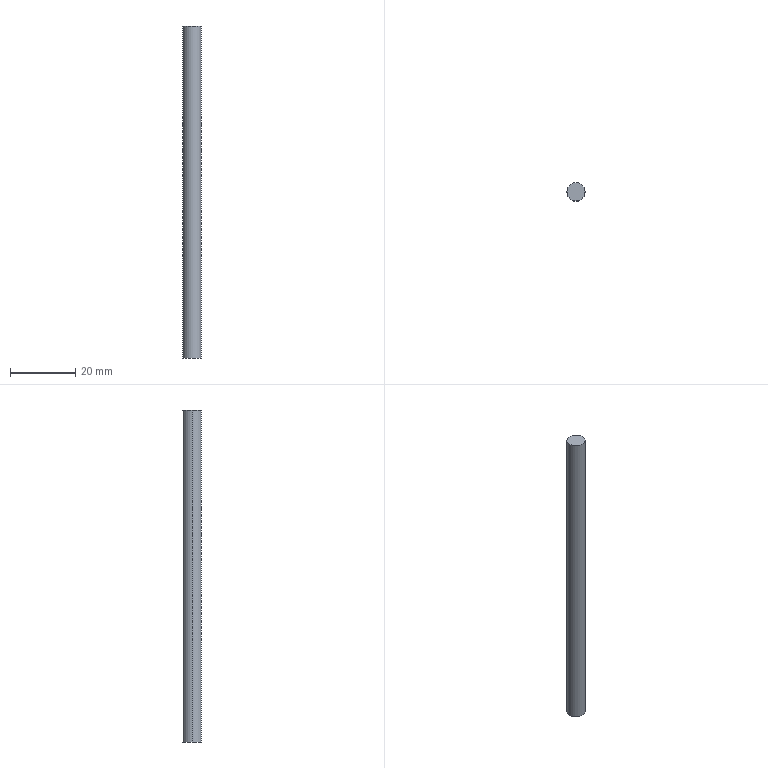Part | SolidWorks | features Extrusion 1 | 1 solid | 4 faces | box 5.6 x 5.6 x 102 mm | volume 2512 mm3 | cylinder 2 | plane 2 | commonest cylinder face diameters 5.6 x2
STEP:
#1=CARTESIAN_POINT('',(-32.2,4.7,-102.));
#2=VERTEX_POINT('',#1);
#3=CARTESIAN_POINT('',(-37.8,4.7,-102.));
#4=VERTEX_POINT('',#3);
#5=CARTESIAN_POINT('',(-35.,4.7,-102.));
#6=DIRECTION('',(0.,0.,1.));
#7=DIRECTION('',(1.,0.,0.));
#8=AXIS2_PLACEMENT_3D('',#5,#6,#7);
#9=CIRCLE('',#8,2.8);
#10=EDGE_CURVE('',#2,#4,#9,.T.);
#11=ORIENTED_EDGE('',*,*,#10,.T.);
#12=CARTESIAN_POINT('',(-37.8,4.7,0.));
#13=VERTEX_POINT('',#12);
#14=CARTESIAN_POINT('',(-37.8,4.7,-102.));
#15=DIRECTION('',(0.,0.,1.));
#16=VECTOR('',#15,1000.);
#17=LINE('',#14,#16);
#18=EDGE_CURVE('',#4,#13,#17,.T.);
#19=ORIENTED_EDGE('',*,*,#18,.T.);
#20=CARTESIAN_POINT('',(-32.2,4.7,0.));
#21=VERTEX_POINT('',#20);
#22=CARTESIAN_POINT('',(-35.,4.7,0.));
#23=DIRECTION('',(0.,0.,1.));
#24=DIRECTION('',(1.,0.,0.));
#25=AXIS2_PLACEMENT_3D('',#22,#23,#24);
#26=CIRCLE('',#25,2.8);
#27=EDGE_CURVE('',#21,#13,#26,.T.);
#28=ORIENTED_EDGE('',*,*,#27,.F.);
#29=CARTESIAN_POINT('',(-32.2,4.7,-102.));
#30=DIRECTION('',(0.,0.,1.));
#31=VECTOR('',#30,1000.);
#32=LINE('',#29,#31);
#33=EDGE_CURVE('',#2,#21,#32,.T.);
#34=ORIENTED_EDGE('',*,*,#33,.F.);
#35=EDGE_LOOP('',(#11,#19,#28,#34));
#36=FACE_OUTER_BOUND('',#35,.T.);
#37=CARTESIAN_POINT('',(-35.,4.7,-102.));
#38=DIRECTION('',(0.,0.,1.));
#39=DIRECTION('',(1.,0.,0.));
#40=AXIS2_PLACEMENT_3D('',#37,#38,#39);
#41=CYLINDRICAL_SURFACE('',#40,2.8);
#42=ADVANCED_FACE('',(#36),#41,.T.);
#43=ORIENTED_EDGE('',*,*,#18,.F.);
#44=CARTESIAN_POINT('',(-35.,4.7,-102.));
#45=DIRECTION('',(0.,0.,1.));
#46=DIRECTION('',(1.,0.,0.));
#47=AXIS2_PLACEMENT_3D('',#44,#45,#46);
#48=CIRCLE('',#47,2.8);
#49=EDGE_CURVE('',#4,#2,#48,.T.);
#50=ORIENTED_EDGE('',*,*,#49,.T.);
#51=ORIENTED_EDGE('',*,*,#33,.T.);
#52=CARTESIAN_POINT('',(-35.,4.7,0.));
#53=DIRECTION('',(0.,0.,1.));
#54=DIRECTION('',(1.,0.,0.));
#55=AXIS2_PLACEMENT_3D('',#52,#53,#54);
#56=CIRCLE('',#55,2.8);
#57=EDGE_CURVE('',#13,#21,#56,.T.);
#58=ORIENTED_EDGE('',*,*,#57,.F.);
#59=EDGE_LOOP('',(#43,#50,#51,#58));
#60=FACE_OUTER_BOUND('',#59,.T.);
#61=CARTESIAN_POINT('',(-35.,4.7,-102.));
#62=DIRECTION('',(0.,0.,1.));
#63=DIRECTION('',(1.,0.,0.));
#64=AXIS2_PLACEMENT_3D('',#61,#62,#63);
#65=CYLINDRICAL_SURFACE('',#64,2.8);
#66=ADVANCED_FACE('',(#60),#65,.T.);
#67=ORIENTED_EDGE('',*,*,#10,.F.);
#68=ORIENTED_EDGE('',*,*,#49,.F.);
#69=EDGE_LOOP('',(#67,#68));
#70=FACE_OUTER_BOUND('',#69,.T.);
#71=CARTESIAN_POINT('',(-35.,4.7,-102.));
#72=DIRECTION('',(0.,0.,1.));
#73=DIRECTION('',(1.,0.,0.));
#74=AXIS2_PLACEMENT_3D('',#71,#72,#73);
#75=PLANE('',#74);
#76=ADVANCED_FACE('',(#70),#75,.F.);
#77=ORIENTED_EDGE('',*,*,#27,.T.);
#78=ORIENTED_EDGE('',*,*,#57,.T.);
#79=EDGE_LOOP('',(#77,#78));
#80=FACE_OUTER_BOUND('',#79,.T.);
#81=CARTESIAN_POINT('',(-35.,4.7,0.));
#82=DIRECTION('',(0.,0.,1.));
#83=DIRECTION('',(1.,0.,0.));
#84=AXIS2_PLACEMENT_3D('',#81,#82,#83);
#85=PLANE('',#84);
#86=ADVANCED_FACE('',(#80),#85,.T.);
#87=CLOSED_SHELL('',(#42,#66,#76,#86));
#88=MANIFOLD_SOLID_BREP('',#87);
#89=CARTESIAN_POINT('',(0.,0.,0.));
#90=DIRECTION('',(0.,0.,1.));
#91=DIRECTION('',(1.,0.,0.));
#92=AXIS2_PLACEMENT_3D('',#89,#90,#91);
#93=(LENGTH_UNIT()NAMED_UNIT(*)SI_UNIT(.MILLI.,.METRE.));
#94=UNCERTAINTY_MEASURE_WITH_UNIT(LENGTH_MEASURE(0.00001),#93,'','');
#95=(NAMED_UNIT(*)PLANE_ANGLE_UNIT()SI_UNIT($,.RADIAN.));
#96=(NAMED_UNIT(*)SI_UNIT($,.STERADIAN.)SOLID_ANGLE_UNIT());
#97=(GEOMETRIC_REPRESENTATION_CONTEXT(3)GLOBAL_UNCERTAINTY_ASSIGNED_CONTEXT((#94))GLOBAL_UNIT_ASSIGNED_CONTEXT((#93,#95,#96))REPRESENTATION_CONTEXT('',''));
#98=ADVANCED_BREP_SHAPE_REPRESENTATION('',(#88,#92),#97);